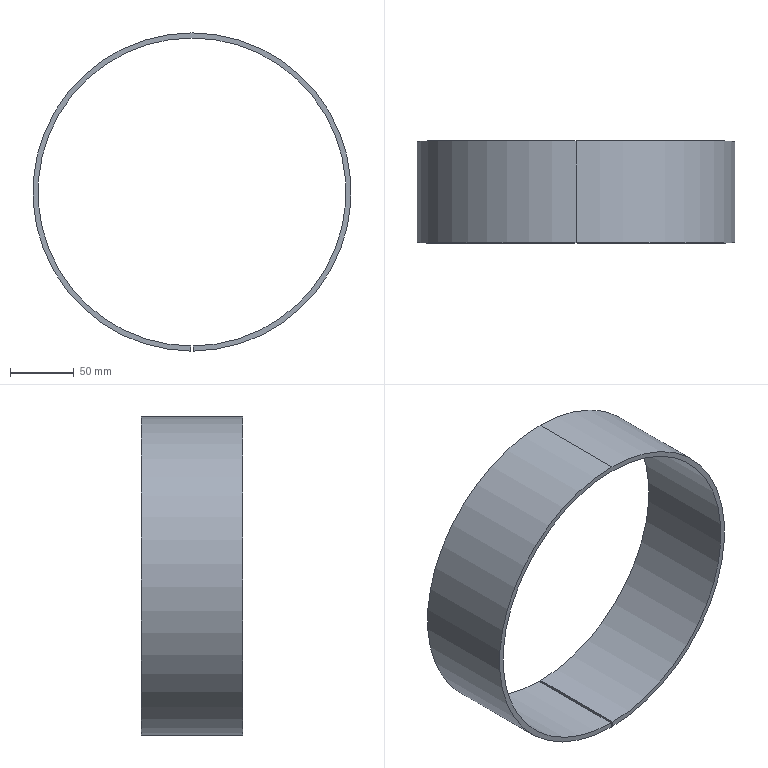Part | SolidWorks | features FlatPattern 1, SheetMetal 1, SweptFlange 1 | 1 solid | 8 faces | box 250 x 80 x 249.996 mm | volume 246676 mm3 | cylinder 4 | plane 4 | commonest cylinder face diameters 242 x2 250 x2
STEP:
#1=CARTESIAN_POINT('',(-1.,0.,-124.996));
#2=VERTEX_POINT('',#1);
#3=CARTESIAN_POINT('',(0.,0.,125.));
#4=VERTEX_POINT('',#3);
#5=CARTESIAN_POINT('',(0.,0.,0.));
#6=DIRECTION('',(0.,1.,0.));
#7=DIRECTION('',(0.,0.,1.));
#8=AXIS2_PLACEMENT_3D('',#5,#6,#7);
#9=CIRCLE('',#8,125.);
#10=EDGE_CURVE('',#2,#4,#9,.T.);
#11=ORIENTED_EDGE('',*,*,#10,.T.);
#12=CARTESIAN_POINT('',(0.,80.,125.));
#13=VERTEX_POINT('',#12);
#14=CARTESIAN_POINT('',(0.,0.,125.));
#15=DIRECTION('',(0.,1.,0.));
#16=VECTOR('',#15,1000.);
#17=LINE('',#14,#16);
#18=EDGE_CURVE('',#4,#13,#17,.T.);
#19=ORIENTED_EDGE('',*,*,#18,.T.);
#20=CARTESIAN_POINT('',(-1.,80.,-124.996));
#21=VERTEX_POINT('',#20);
#22=CARTESIAN_POINT('',(0.,80.,0.));
#23=DIRECTION('',(0.,1.,0.));
#24=DIRECTION('',(0.,0.,1.));
#25=AXIS2_PLACEMENT_3D('',#22,#23,#24);
#26=CIRCLE('',#25,125.);
#27=EDGE_CURVE('',#21,#13,#26,.T.);
#28=ORIENTED_EDGE('',*,*,#27,.F.);
#29=CARTESIAN_POINT('',(-1.,0.,-124.996));
#30=DIRECTION('',(0.,1.,0.));
#31=VECTOR('',#30,1000.);
#32=LINE('',#29,#31);
#33=EDGE_CURVE('',#2,#21,#32,.T.);
#34=ORIENTED_EDGE('',*,*,#33,.F.);
#35=EDGE_LOOP('',(#11,#19,#28,#34));
#36=FACE_OUTER_BOUND('',#35,.T.);
#37=CARTESIAN_POINT('',(0.,0.,0.));
#38=DIRECTION('',(0.,1.,0.));
#39=DIRECTION('',(0.,0.,1.));
#40=AXIS2_PLACEMENT_3D('',#37,#38,#39);
#41=CYLINDRICAL_SURFACE('',#40,125.);
#42=ADVANCED_FACE('',(#36),#41,.T.);
#43=CARTESIAN_POINT('',(0.,0.,121.));
#44=VERTEX_POINT('',#43);
#45=CARTESIAN_POINT('',(0.968,0.,-120.996));
#46=VERTEX_POINT('',#45);
#47=CARTESIAN_POINT('',(0.,0.,0.));
#48=DIRECTION('',(0.,1.,0.));
#49=DIRECTION('',(0.,0.,1.));
#50=AXIS2_PLACEMENT_3D('',#47,#48,#49);
#51=CIRCLE('',#50,121.);
#52=EDGE_CURVE('',#44,#46,#51,.T.);
#53=ORIENTED_EDGE('',*,*,#52,.F.);
#54=CARTESIAN_POINT('',(0.,80.,121.));
#55=VERTEX_POINT('',#54);
#56=CARTESIAN_POINT('',(0.,0.,121.));
#57=DIRECTION('',(0.,1.,0.));
#58=VECTOR('',#57,1000.);
#59=LINE('',#56,#58);
#60=EDGE_CURVE('',#44,#55,#59,.T.);
#61=ORIENTED_EDGE('',*,*,#60,.T.);
#62=CARTESIAN_POINT('',(0.968,80.,-120.996));
#63=VERTEX_POINT('',#62);
#64=CARTESIAN_POINT('',(0.,80.,0.));
#65=DIRECTION('',(0.,1.,0.));
#66=DIRECTION('',(0.,0.,1.));
#67=AXIS2_PLACEMENT_3D('',#64,#65,#66);
#68=CIRCLE('',#67,121.);
#69=EDGE_CURVE('',#55,#63,#68,.T.);
#70=ORIENTED_EDGE('',*,*,#69,.T.);
#71=CARTESIAN_POINT('',(0.968,0.,-120.996));
#72=DIRECTION('',(0.,1.,0.));
#73=VECTOR('',#72,1000.);
#74=LINE('',#71,#73);
#75=EDGE_CURVE('',#46,#63,#74,.T.);
#76=ORIENTED_EDGE('',*,*,#75,.F.);
#77=EDGE_LOOP('',(#53,#61,#70,#76));
#78=FACE_OUTER_BOUND('',#77,.T.);
#79=CARTESIAN_POINT('',(0.,0.,0.));
#80=DIRECTION('',(0.,1.,0.));
#81=DIRECTION('',(0.,0.,1.));
#82=AXIS2_PLACEMENT_3D('',#79,#80,#81);
#83=CYLINDRICAL_SURFACE('',#82,121.);
#84=ADVANCED_FACE('',(#78),#83,.F.);
#85=CARTESIAN_POINT('',(-0.968,0.,-120.996));
#86=VERTEX_POINT('',#85);
#87=CARTESIAN_POINT('',(-1.,0.,-124.996));
#88=DIRECTION('',(0.008,0.,1.));
#89=VECTOR('',#88,1000.);
#90=LINE('',#87,#89);
#91=EDGE_CURVE('',#2,#86,#90,.T.);
#92=ORIENTED_EDGE('',*,*,#91,.F.);
#93=ORIENTED_EDGE('',*,*,#33,.T.);
#94=CARTESIAN_POINT('',(-0.968,80.,-120.996));
#95=VERTEX_POINT('',#94);
#96=CARTESIAN_POINT('',(-1.,80.,-124.996));
#97=DIRECTION('',(0.008,0.,1.));
#98=VECTOR('',#97,1000.);
#99=LINE('',#96,#98);
#100=EDGE_CURVE('',#21,#95,#99,.T.);
#101=ORIENTED_EDGE('',*,*,#100,.T.);
#102=CARTESIAN_POINT('',(-0.968,0.,-120.996));
#103=DIRECTION('',(0.,1.,0.));
#104=VECTOR('',#103,1000.);
#105=LINE('',#102,#104);
#106=EDGE_CURVE('',#86,#95,#105,.T.);
#107=ORIENTED_EDGE('',*,*,#106,.F.);
#108=EDGE_LOOP('',(#92,#93,#101,#107));
#109=FACE_OUTER_BOUND('',#108,.T.);
#110=CARTESIAN_POINT('',(-1.,40.,-124.996));
#111=DIRECTION('',(-1.,0.,0.008));
#112=DIRECTION('',(0.,1.,0.));
#113=AXIS2_PLACEMENT_3D('',#110,#111,#112);
#114=PLANE('',#113);
#115=ADVANCED_FACE('',(#109),#114,.F.);
#116=ORIENTED_EDGE('',*,*,#100,.F.);
#117=ORIENTED_EDGE('',*,*,#27,.T.);
#118=CARTESIAN_POINT('',(1.,80.,-124.996));
#119=VERTEX_POINT('',#118);
#120=CARTESIAN_POINT('',(0.,80.,0.));
#121=DIRECTION('',(0.,1.,0.));
#122=DIRECTION('',(0.,0.,1.));
#123=AXIS2_PLACEMENT_3D('',#120,#121,#122);
#124=CIRCLE('',#123,125.);
#125=EDGE_CURVE('',#13,#119,#124,.T.);
#126=ORIENTED_EDGE('',*,*,#125,.T.);
#127=CARTESIAN_POINT('',(1.,80.,-124.996));
#128=DIRECTION('',(-0.008,0.,1.));
#129=VECTOR('',#128,1000.);
#130=LINE('',#127,#129);
#131=EDGE_CURVE('',#119,#63,#130,.T.);
#132=ORIENTED_EDGE('',*,*,#131,.T.);
#133=ORIENTED_EDGE('',*,*,#69,.F.);
#134=CARTESIAN_POINT('',(0.,80.,0.));
#135=DIRECTION('',(0.,1.,0.));
#136=DIRECTION('',(0.,0.,1.));
#137=AXIS2_PLACEMENT_3D('',#134,#135,#136);
#138=CIRCLE('',#137,121.);
#139=EDGE_CURVE('',#95,#55,#138,.T.);
#140=ORIENTED_EDGE('',*,*,#139,.F.);
#141=EDGE_LOOP('',(#116,#117,#126,#132,#133,#140));
#142=FACE_OUTER_BOUND('',#141,.T.);
#143=CARTESIAN_POINT('',(0.,80.,0.));
#144=DIRECTION('',(0.,-1.,0.));
#145=DIRECTION('',(0.,0.,-1.));
#146=AXIS2_PLACEMENT_3D('',#143,#144,#145);
#147=PLANE('',#146);
#148=ADVANCED_FACE('',(#142),#147,.F.);
#149=ORIENTED_EDGE('',*,*,#131,.F.);
#150=CARTESIAN_POINT('',(1.,0.,-124.996));
#151=VERTEX_POINT('',#150);
#152=CARTESIAN_POINT('',(1.,0.,-124.996));
#153=DIRECTION('',(0.,1.,0.));
#154=VECTOR('',#153,1000.);
#155=LINE('',#152,#154);
#156=EDGE_CURVE('',#151,#119,#155,.T.);
#157=ORIENTED_EDGE('',*,*,#156,.F.);
#158=CARTESIAN_POINT('',(1.,0.,-124.996));
#159=DIRECTION('',(-0.008,0.,1.));
#160=VECTOR('',#159,1000.);
#161=LINE('',#158,#160);
#162=EDGE_CURVE('',#151,#46,#161,.T.);
#163=ORIENTED_EDGE('',*,*,#162,.T.);
#164=ORIENTED_EDGE('',*,*,#75,.T.);
#165=EDGE_LOOP('',(#149,#157,#163,#164));
#166=FACE_OUTER_BOUND('',#165,.T.);
#167=CARTESIAN_POINT('',(1.,40.,-124.996));
#168=DIRECTION('',(-1.,0.,-0.008));
#169=DIRECTION('',(0.,1.,0.));
#170=AXIS2_PLACEMENT_3D('',#167,#168,#169);
#171=PLANE('',#170);
#172=ADVANCED_FACE('',(#166),#171,.T.);
#173=ORIENTED_EDGE('',*,*,#10,.F.);
#174=ORIENTED_EDGE('',*,*,#91,.T.);
#175=CARTESIAN_POINT('',(0.,0.,0.));
#176=DIRECTION('',(0.,1.,0.));
#177=DIRECTION('',(0.,0.,1.));
#178=AXIS2_PLACEMENT_3D('',#175,#176,#177);
#179=CIRCLE('',#178,121.);
#180=EDGE_CURVE('',#86,#44,#179,.T.);
#181=ORIENTED_EDGE('',*,*,#180,.T.);
#182=ORIENTED_EDGE('',*,*,#52,.T.);
#183=ORIENTED_EDGE('',*,*,#162,.F.);
#184=CARTESIAN_POINT('',(0.,0.,0.));
#185=DIRECTION('',(0.,1.,0.));
#186=DIRECTION('',(0.,0.,1.));
#187=AXIS2_PLACEMENT_3D('',#184,#185,#186);
#188=CIRCLE('',#187,125.);
#189=EDGE_CURVE('',#4,#151,#188,.T.);
#190=ORIENTED_EDGE('',*,*,#189,.F.);
#191=EDGE_LOOP('',(#173,#174,#181,#182,#183,#190));
#192=FACE_OUTER_BOUND('',#191,.T.);
#193=CARTESIAN_POINT('',(0.,0.,0.));
#194=DIRECTION('',(0.,-1.,0.));
#195=DIRECTION('',(0.,0.,-1.));
#196=AXIS2_PLACEMENT_3D('',#193,#194,#195);
#197=PLANE('',#196);
#198=ADVANCED_FACE('',(#192),#197,.T.);
#199=ORIENTED_EDGE('',*,*,#60,.F.);
#200=ORIENTED_EDGE('',*,*,#180,.F.);
#201=ORIENTED_EDGE('',*,*,#106,.T.);
#202=ORIENTED_EDGE('',*,*,#139,.T.);
#203=EDGE_LOOP('',(#199,#200,#201,#202));
#204=FACE_OUTER_BOUND('',#203,.T.);
#205=CARTESIAN_POINT('',(0.,0.,0.));
#206=DIRECTION('',(0.,1.,0.));
#207=DIRECTION('',(0.,0.,1.));
#208=AXIS2_PLACEMENT_3D('',#205,#206,#207);
#209=CYLINDRICAL_SURFACE('',#208,121.);
#210=ADVANCED_FACE('',(#204),#209,.F.);
#211=ORIENTED_EDGE('',*,*,#18,.F.);
#212=ORIENTED_EDGE('',*,*,#189,.T.);
#213=ORIENTED_EDGE('',*,*,#156,.T.);
#214=ORIENTED_EDGE('',*,*,#125,.F.);
#215=EDGE_LOOP('',(#211,#212,#213,#214));
#216=FACE_OUTER_BOUND('',#215,.T.);
#217=CARTESIAN_POINT('',(0.,0.,0.));
#218=DIRECTION('',(0.,1.,0.));
#219=DIRECTION('',(0.,0.,1.));
#220=AXIS2_PLACEMENT_3D('',#217,#218,#219);
#221=CYLINDRICAL_SURFACE('',#220,125.);
#222=ADVANCED_FACE('',(#216),#221,.T.);
#223=CLOSED_SHELL('',(#42,#84,#115,#148,#172,#198,#210,#222));
#224=MANIFOLD_SOLID_BREP('',#223);
#225=CARTESIAN_POINT('',(0.,0.,0.));
#226=DIRECTION('',(0.,0.,1.));
#227=DIRECTION('',(1.,0.,0.));
#228=AXIS2_PLACEMENT_3D('',#225,#226,#227);
#229=(LENGTH_UNIT()NAMED_UNIT(*)SI_UNIT(.MILLI.,.METRE.));
#230=UNCERTAINTY_MEASURE_WITH_UNIT(LENGTH_MEASURE(0.00001),#229,'','');
#231=(NAMED_UNIT(*)PLANE_ANGLE_UNIT()SI_UNIT($,.RADIAN.));
#232=(NAMED_UNIT(*)SI_UNIT($,.STERADIAN.)SOLID_ANGLE_UNIT());
#233=(GEOMETRIC_REPRESENTATION_CONTEXT(3)GLOBAL_UNCERTAINTY_ASSIGNED_CONTEXT((#230))GLOBAL_UNIT_ASSIGNED_CONTEXT((#229,#231,#232))REPRESENTATION_CONTEXT('',''));
#234=ADVANCED_BREP_SHAPE_REPRESENTATION('',(#224,#228),#233);